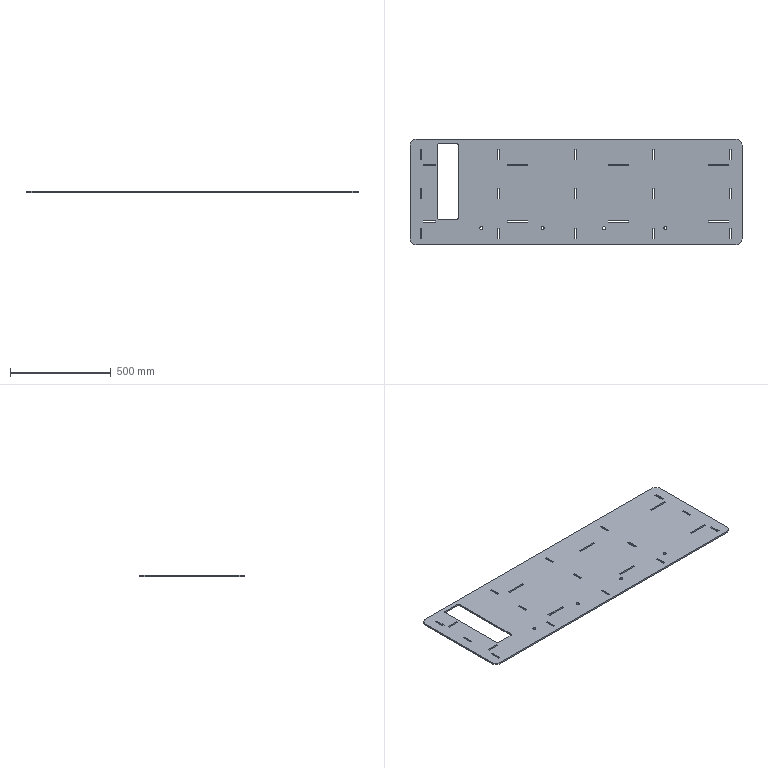Part | SolidWorks | features FlatPattern 1, SMBaseFlange 1, SheetMetal 1 | 1 solid | 118 faces | box 1650 x 525 x 8 mm | volume 6516839 mm3 | plane 102 | cylinder 16 | commonest cylinder face diameters 15 x12 60 x4